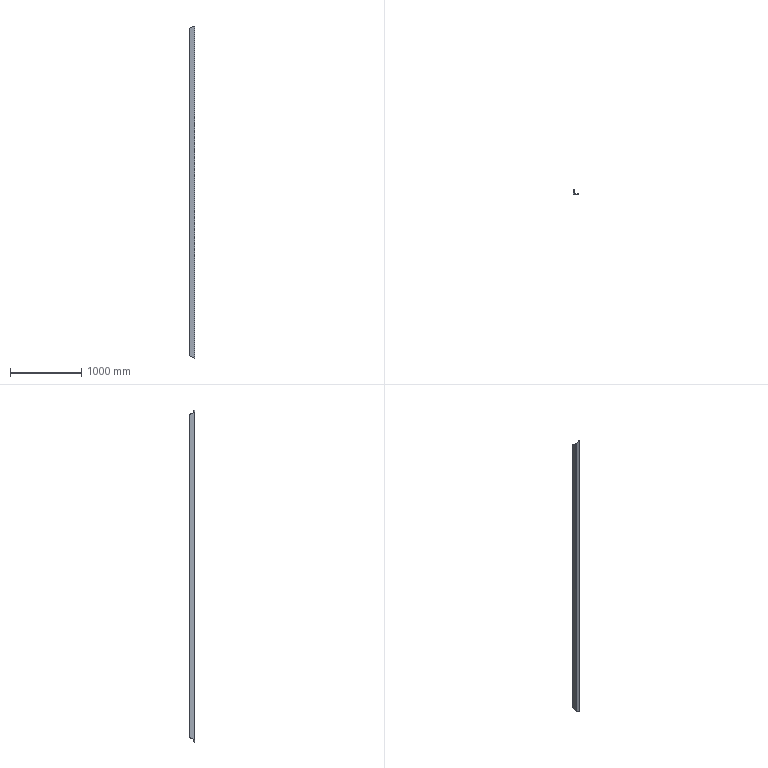Part | SolidWorks | features Extrusion 1, ICE 1 | 1 solid | 11 faces | box 70 x 70 x 4645 mm | volume 4877091 mm3 | plane 8 | cylinder 3 | commonest cylinder face diameters 6 x2 16 x1
STEP:
#1=CARTESIAN_POINT('',(5.,70.,4578.159));
#2=VERTEX_POINT('',#1);
#3=CARTESIAN_POINT('',(0.,70.,4575.683));
#4=VERTEX_POINT('',#3);
#5=CARTESIAN_POINT('',(31.579,70.,4591.318));
#6=DIRECTION('',(-0.8962,0.,-0.4437));
#7=VECTOR('',#6,1000.);
#8=LINE('',#5,#7);
#9=EDGE_CURVE('',#2,#4,#8,.T.);
#10=ORIENTED_EDGE('',*,*,#9,.F.);
#11=CARTESIAN_POINT('',(5.,70.,66.841));
#12=VERTEX_POINT('',#11);
#13=CARTESIAN_POINT('',(5.,70.,4645.));
#14=DIRECTION('',(0.,0.,-1.));
#15=VECTOR('',#14,1000.);
#16=LINE('',#13,#15);
#17=EDGE_CURVE('',#2,#12,#16,.T.);
#18=ORIENTED_EDGE('',*,*,#17,.T.);
#19=CARTESIAN_POINT('',(0.,70.,69.317));
#20=VERTEX_POINT('',#19);
#21=CARTESIAN_POINT('',(-1815.466,70.,968.193));
#22=DIRECTION('',(0.8962,0.,-0.4437));
#23=VECTOR('',#22,1000.);
#24=LINE('',#21,#23);
#25=EDGE_CURVE('',#20,#12,#24,.T.);
#26=ORIENTED_EDGE('',*,*,#25,.F.);
#27=CARTESIAN_POINT('',(0.,70.,4645.));
#28=DIRECTION('',(0.,0.,-1.));
#29=VECTOR('',#28,1000.);
#30=LINE('',#27,#29);
#31=EDGE_CURVE('',#4,#20,#30,.T.);
#32=ORIENTED_EDGE('',*,*,#31,.F.);
#33=EDGE_LOOP('',(#10,#18,#26,#32));
#34=FACE_OUTER_BOUND('',#33,.T.);
#35=CARTESIAN_POINT('',(5.,70.,4645.));
#36=DIRECTION('',(0.,-1.,0.));
#37=DIRECTION('',(0.,0.,-1.));
#38=AXIS2_PLACEMENT_3D('',#35,#36,#37);
#39=PLANE('',#38);
#40=ADVANCED_FACE('',(#34),#39,.F.);
#41=CARTESIAN_POINT('',(0.,0.,4610.341));
#42=VERTEX_POINT('',#41);
#43=CARTESIAN_POINT('',(0.,42.437,4589.33));
#44=DIRECTION('',(0.,-0.8962,0.4437));
#45=VECTOR('',#44,1000.);
#46=LINE('',#43,#45);
#47=EDGE_CURVE('',#4,#42,#46,.T.);
#48=ORIENTED_EDGE('',*,*,#47,.F.);
#49=ORIENTED_EDGE('',*,*,#31,.T.);
#50=CARTESIAN_POINT('',(0.,0.,34.659));
#51=VERTEX_POINT('',#50);
#52=CARTESIAN_POINT('',(0.,1889.482,970.181));
#53=DIRECTION('',(0.,0.8962,0.4437));
#54=VECTOR('',#53,1000.);
#55=LINE('',#52,#54);
#56=EDGE_CURVE('',#51,#20,#55,.T.);
#57=ORIENTED_EDGE('',*,*,#56,.F.);
#58=CARTESIAN_POINT('',(0.,0.,4645.));
#59=DIRECTION('',(0.,0.,-1.));
#60=VECTOR('',#59,1000.);
#61=LINE('',#58,#60);
#62=EDGE_CURVE('',#42,#51,#61,.T.);
#63=ORIENTED_EDGE('',*,*,#62,.F.);
#64=EDGE_LOOP('',(#48,#49,#57,#63));
#65=FACE_OUTER_BOUND('',#64,.T.);
#66=CARTESIAN_POINT('',(0.,70.,4645.));
#67=DIRECTION('',(1.,0.,0.));
#68=DIRECTION('',(0.,0.,-1.));
#69=AXIS2_PLACEMENT_3D('',#66,#67,#68);
#70=PLANE('',#69);
#71=ADVANCED_FACE('',(#65),#70,.F.);
#72=CARTESIAN_POINT('',(70.,0.,4645.));
#73=VERTEX_POINT('',#72);
#74=CARTESIAN_POINT('',(13.782,0.,4617.165));
#75=DIRECTION('',(0.8962,0.,0.4437));
#76=VECTOR('',#75,1000.);
#77=LINE('',#74,#76);
#78=EDGE_CURVE('',#42,#73,#77,.T.);
#79=ORIENTED_EDGE('',*,*,#78,.F.);
#80=ORIENTED_EDGE('',*,*,#62,.T.);
#81=CARTESIAN_POINT('',(70.,0.,0.));
#82=VERTEX_POINT('',#81);
#83=CARTESIAN_POINT('',(-1833.263,0.,942.347));
#84=DIRECTION('',(-0.8962,0.,0.4437));
#85=VECTOR('',#84,1000.);
#86=LINE('',#83,#85);
#87=EDGE_CURVE('',#82,#51,#86,.T.);
#88=ORIENTED_EDGE('',*,*,#87,.F.);
#89=CARTESIAN_POINT('',(70.,0.,4645.));
#90=DIRECTION('',(0.,0.,-1.));
#91=VECTOR('',#90,1000.);
#92=LINE('',#89,#91);
#93=EDGE_CURVE('',#73,#82,#92,.T.);
#94=ORIENTED_EDGE('',*,*,#93,.F.);
#95=EDGE_LOOP('',(#79,#80,#88,#94));
#96=FACE_OUTER_BOUND('',#95,.T.);
#97=CARTESIAN_POINT('',(0.,0.,4645.));
#98=DIRECTION('',(0.,1.,0.));
#99=DIRECTION('',(0.,0.,1.));
#100=AXIS2_PLACEMENT_3D('',#97,#98,#99);
#101=PLANE('',#100);
#102=ADVANCED_FACE('',(#96),#101,.F.);
#103=CARTESIAN_POINT('',(70.,5.,4642.524));
#104=VERTEX_POINT('',#103);
#105=CARTESIAN_POINT('',(70.,0.,4645.));
#106=DIRECTION('',(0.,0.8962,-0.4437));
#107=VECTOR('',#106,1000.);
#108=LINE('',#105,#107);
#109=EDGE_CURVE('',#73,#104,#108,.T.);
#110=ORIENTED_EDGE('',*,*,#109,.F.);
#111=ORIENTED_EDGE('',*,*,#93,.T.);
#112=CARTESIAN_POINT('',(70.,5.,2.476));
#113=VERTEX_POINT('',#112);
#114=CARTESIAN_POINT('',(70.,1847.045,914.512));
#115=DIRECTION('',(0.,-0.8962,-0.4437));
#116=VECTOR('',#115,1000.);
#117=LINE('',#114,#116);
#118=EDGE_CURVE('',#113,#82,#117,.T.);
#119=ORIENTED_EDGE('',*,*,#118,.F.);
#120=CARTESIAN_POINT('',(70.,5.,4645.));
#121=DIRECTION('',(0.,0.,-1.));
#122=VECTOR('',#121,1000.);
#123=LINE('',#120,#122);
#124=EDGE_CURVE('',#104,#113,#123,.T.);
#125=ORIENTED_EDGE('',*,*,#124,.F.);
#126=EDGE_LOOP('',(#110,#111,#119,#125));
#127=FACE_OUTER_BOUND('',#126,.T.);
#128=CARTESIAN_POINT('',(70.,0.,4645.));
#129=DIRECTION('',(-1.,0.,0.));
#130=DIRECTION('',(0.,0.,1.));
#131=AXIS2_PLACEMENT_3D('',#128,#129,#130);
#132=PLANE('',#131);
#133=ADVANCED_FACE('',(#127),#132,.F.);
#134=CARTESIAN_POINT('',(67.,8.,4639.554));
#135=VERTEX_POINT('',#134);
#136=CARTESIAN_POINT('',(70.,5.,4642.524));
#137=CARTESIAN_POINT('',(70.,6.757,4641.654));
#138=CARTESIAN_POINT('',(68.757,8.,4640.424));
#139=CARTESIAN_POINT('',(67.,8.,4639.554));
#140=(BOUNDED_CURVE()B_SPLINE_CURVE(3,(#136,#137,#138,#139),.UNSPECIFIED.,.F.,.F.)B_SPLINE_CURVE_WITH_KNOTS((4,4),(3.927,5.498),.UNSPECIFIED.)CURVE()GEOMETRIC_REPRESENTATION_ITEM()RATIONAL_B_SPLINE_CURVE((1.,0.8047,0.8047,1.))REPRESENTATION_ITEM(''));
#141=EDGE_CURVE('',#104,#135,#140,.T.);
#142=ORIENTED_EDGE('',*,*,#141,.F.);
#143=ORIENTED_EDGE('',*,*,#124,.T.);
#144=CARTESIAN_POINT('',(67.,8.,5.446));
#145=VERTEX_POINT('',#144);
#146=CARTESIAN_POINT('',(67.,8.,5.446));
#147=CARTESIAN_POINT('',(68.757,8.,4.576));
#148=CARTESIAN_POINT('',(70.,6.757,3.346));
#149=CARTESIAN_POINT('',(70.,5.,2.476));
#150=(BOUNDED_CURVE()B_SPLINE_CURVE(3,(#146,#147,#148,#149),.UNSPECIFIED.,.F.,.F.)B_SPLINE_CURVE_WITH_KNOTS((4,4),(3.927,5.498),.UNSPECIFIED.)CURVE()GEOMETRIC_REPRESENTATION_ITEM()RATIONAL_B_SPLINE_CURVE((1.,0.8047,0.8047,1.))REPRESENTATION_ITEM(''));
#151=EDGE_CURVE('',#145,#113,#150,.T.);
#152=ORIENTED_EDGE('',*,*,#151,.F.);
#153=CARTESIAN_POINT('',(67.,8.,4645.));
#154=DIRECTION('',(0.,0.,-1.));
#155=VECTOR('',#154,1000.);
#156=LINE('',#153,#155);
#157=EDGE_CURVE('',#135,#145,#156,.T.);
#158=ORIENTED_EDGE('',*,*,#157,.F.);
#159=EDGE_LOOP('',(#142,#143,#152,#158));
#160=FACE_OUTER_BOUND('',#159,.T.);
#161=CARTESIAN_POINT('',(67.,5.,4645.));
#162=DIRECTION('',(0.,0.,-1.));
#163=DIRECTION('',(-1.,0.,0.));
#164=AXIS2_PLACEMENT_3D('',#161,#162,#163);
#165=CYLINDRICAL_SURFACE('',#164,3.);
#166=ADVANCED_FACE('',(#160),#165,.T.);
#167=CARTESIAN_POINT('',(16.,8.,4614.302));
#168=VERTEX_POINT('',#167);
#169=CARTESIAN_POINT('',(69.166,8.,4640.626));
#170=DIRECTION('',(-0.8962,0.,-0.4437));
#171=VECTOR('',#170,1000.);
#172=LINE('',#169,#171);
#173=EDGE_CURVE('',#135,#168,#172,.T.);
#174=ORIENTED_EDGE('',*,*,#173,.F.);
#175=ORIENTED_EDGE('',*,*,#157,.T.);
#176=CARTESIAN_POINT('',(16.,8.,30.698));
#177=VERTEX_POINT('',#176);
#178=CARTESIAN_POINT('',(-1777.879,8.,918.886));
#179=DIRECTION('',(0.8962,0.,-0.4437));
#180=VECTOR('',#179,1000.);
#181=LINE('',#178,#180);
#182=EDGE_CURVE('',#177,#145,#181,.T.);
#183=ORIENTED_EDGE('',*,*,#182,.F.);
#184=CARTESIAN_POINT('',(16.,8.,4645.));
#185=DIRECTION('',(0.,0.,-1.));
#186=VECTOR('',#185,1000.);
#187=LINE('',#184,#186);
#188=EDGE_CURVE('',#168,#177,#187,.T.);
#189=ORIENTED_EDGE('',*,*,#188,.F.);
#190=EDGE_LOOP('',(#174,#175,#183,#189));
#191=FACE_OUTER_BOUND('',#190,.T.);
#192=CARTESIAN_POINT('',(67.,8.,4645.));
#193=DIRECTION('',(0.,-1.,0.));
#194=DIRECTION('',(1.,0.,0.));
#195=AXIS2_PLACEMENT_3D('',#192,#193,#194);
#196=PLANE('',#195);
#197=ADVANCED_FACE('',(#191),#196,.F.);
#198=CARTESIAN_POINT('',(8.,16.,4606.381));
#199=VERTEX_POINT('',#198);
#200=CARTESIAN_POINT('',(16.,8.,4614.302));
#201=CARTESIAN_POINT('',(11.314,8.,4611.982));
#202=CARTESIAN_POINT('',(8.,11.314,4608.701));
#203=CARTESIAN_POINT('',(8.,16.,4606.381));
#204=(BOUNDED_CURVE()B_SPLINE_CURVE(3,(#200,#201,#202,#203),.UNSPECIFIED.,.F.,.F.)B_SPLINE_CURVE_WITH_KNOTS((4,4),(3.927,5.498),.UNSPECIFIED.)CURVE()GEOMETRIC_REPRESENTATION_ITEM()RATIONAL_B_SPLINE_CURVE((1.,0.8047,0.8047,1.))REPRESENTATION_ITEM(''));
#205=EDGE_CURVE('',#168,#199,#204,.T.);
#206=ORIENTED_EDGE('',*,*,#205,.F.);
#207=ORIENTED_EDGE('',*,*,#188,.T.);
#208=CARTESIAN_POINT('',(8.,16.,38.619));
#209=VERTEX_POINT('',#208);
#210=CARTESIAN_POINT('',(8.,16.,38.619));
#211=CARTESIAN_POINT('',(8.,11.314,36.299));
#212=CARTESIAN_POINT('',(11.314,8.,33.018));
#213=CARTESIAN_POINT('',(16.,8.,30.698));
#214=(BOUNDED_CURVE()B_SPLINE_CURVE(3,(#210,#211,#212,#213),.UNSPECIFIED.,.F.,.F.)B_SPLINE_CURVE_WITH_KNOTS((4,4),(3.927,5.498),.UNSPECIFIED.)CURVE()GEOMETRIC_REPRESENTATION_ITEM()RATIONAL_B_SPLINE_CURVE((1.,0.8047,0.8047,1.))REPRESENTATION_ITEM(''));
#215=EDGE_CURVE('',#209,#177,#214,.T.);
#216=ORIENTED_EDGE('',*,*,#215,.F.);
#217=CARTESIAN_POINT('',(8.,16.,4645.));
#218=DIRECTION('',(0.,0.,-1.));
#219=VECTOR('',#218,1000.);
#220=LINE('',#217,#219);
#221=EDGE_CURVE('',#199,#209,#220,.T.);
#222=ORIENTED_EDGE('',*,*,#221,.F.);
#223=EDGE_LOOP('',(#206,#207,#216,#222));
#224=FACE_OUTER_BOUND('',#223,.T.);
#225=CARTESIAN_POINT('',(16.,16.,4645.));
#226=DIRECTION('',(0.,0.,-1.));
#227=DIRECTION('',(-1.,0.,0.));
#228=AXIS2_PLACEMENT_3D('',#225,#226,#227);
#229=CYLINDRICAL_SURFACE('',#228,8.);
#230=ADVANCED_FACE('',(#224),#229,.F.);
#231=CARTESIAN_POINT('',(8.,67.,4581.129));
#232=VERTEX_POINT('',#231);
#233=CARTESIAN_POINT('',(8.,0.6433,4613.984));
#234=DIRECTION('',(0.,0.8962,-0.4437));
#235=VECTOR('',#234,1000.);
#236=LINE('',#233,#235);
#237=EDGE_CURVE('',#199,#232,#236,.T.);
#238=ORIENTED_EDGE('',*,*,#237,.F.);
#239=ORIENTED_EDGE('',*,*,#221,.T.);
#240=CARTESIAN_POINT('',(8.,67.,63.871));
#241=VERTEX_POINT('',#240);
#242=CARTESIAN_POINT('',(8.,1847.688,945.528));
#243=DIRECTION('',(0.,-0.8962,-0.4437));
#244=VECTOR('',#243,1000.);
#245=LINE('',#242,#244);
#246=EDGE_CURVE('',#241,#209,#245,.T.);
#247=ORIENTED_EDGE('',*,*,#246,.F.);
#248=CARTESIAN_POINT('',(8.,67.,4645.));
#249=DIRECTION('',(0.,0.,-1.));
#250=VECTOR('',#249,1000.);
#251=LINE('',#248,#250);
#252=EDGE_CURVE('',#232,#241,#251,.T.);
#253=ORIENTED_EDGE('',*,*,#252,.F.);
#254=EDGE_LOOP('',(#238,#239,#247,#253));
#255=FACE_OUTER_BOUND('',#254,.T.);
#256=CARTESIAN_POINT('',(8.,16.,4645.));
#257=DIRECTION('',(-1.,0.,0.));
#258=DIRECTION('',(0.,-1.,0.));
#259=AXIS2_PLACEMENT_3D('',#256,#257,#258);
#260=PLANE('',#259);
#261=ADVANCED_FACE('',(#255),#260,.F.);
#262=CARTESIAN_POINT('',(8.,67.,4581.129));
#263=CARTESIAN_POINT('',(8.,68.757,4580.259));
#264=CARTESIAN_POINT('',(6.757,70.,4579.029));
#265=CARTESIAN_POINT('',(5.,70.,4578.159));
#266=(BOUNDED_CURVE()B_SPLINE_CURVE(3,(#262,#263,#264,#265),.UNSPECIFIED.,.F.,.F.)B_SPLINE_CURVE_WITH_KNOTS((4,4),(3.927,5.498),.UNSPECIFIED.)CURVE()GEOMETRIC_REPRESENTATION_ITEM()RATIONAL_B_SPLINE_CURVE((1.,0.8047,0.8047,1.))REPRESENTATION_ITEM(''));
#267=EDGE_CURVE('',#232,#2,#266,.T.);
#268=ORIENTED_EDGE('',*,*,#267,.F.);
#269=ORIENTED_EDGE('',*,*,#252,.T.);
#270=CARTESIAN_POINT('',(5.,70.,66.841));
#271=CARTESIAN_POINT('',(6.757,70.,65.971));
#272=CARTESIAN_POINT('',(8.,68.757,64.741));
#273=CARTESIAN_POINT('',(8.,67.,63.871));
#274=(BOUNDED_CURVE()B_SPLINE_CURVE(3,(#270,#271,#272,#273),.UNSPECIFIED.,.F.,.F.)B_SPLINE_CURVE_WITH_KNOTS((4,4),(3.927,5.498),.UNSPECIFIED.)CURVE()GEOMETRIC_REPRESENTATION_ITEM()RATIONAL_B_SPLINE_CURVE((1.,0.8047,0.8047,1.))REPRESENTATION_ITEM(''));
#275=EDGE_CURVE('',#12,#241,#274,.T.);
#276=ORIENTED_EDGE('',*,*,#275,.F.);
#277=ORIENTED_EDGE('',*,*,#17,.F.);
#278=EDGE_LOOP('',(#268,#269,#276,#277));
#279=FACE_OUTER_BOUND('',#278,.T.);
#280=CARTESIAN_POINT('',(5.,67.,4645.));
#281=DIRECTION('',(0.,0.,-1.));
#282=DIRECTION('',(-1.,0.,0.));
#283=AXIS2_PLACEMENT_3D('',#280,#281,#282);
#284=CYLINDRICAL_SURFACE('',#283,3.);
#285=ADVANCED_FACE('',(#279),#284,.T.);
#286=ORIENTED_EDGE('',*,*,#25,.T.);
#287=ORIENTED_EDGE('',*,*,#275,.T.);
#288=ORIENTED_EDGE('',*,*,#246,.T.);
#289=ORIENTED_EDGE('',*,*,#215,.T.);
#290=ORIENTED_EDGE('',*,*,#182,.T.);
#291=ORIENTED_EDGE('',*,*,#151,.T.);
#292=ORIENTED_EDGE('',*,*,#118,.T.);
#293=ORIENTED_EDGE('',*,*,#87,.T.);
#294=ORIENTED_EDGE('',*,*,#56,.T.);
#295=EDGE_LOOP('',(#286,#287,#288,#289,#290,#291,#292,#293,#294));
#296=FACE_OUTER_BOUND('',#295,.T.);
#297=CARTESIAN_POINT('',(105.,35.,0.));
#298=DIRECTION('',(-0.4056,0.4056,-0.8192));
#299=DIRECTION('',(0.,0.8962,0.4437));
#300=AXIS2_PLACEMENT_3D('',#297,#298,#299);
#301=PLANE('',#300);
#302=ADVANCED_FACE('',(#296),#301,.T.);
#303=ORIENTED_EDGE('',*,*,#9,.T.);
#304=ORIENTED_EDGE('',*,*,#47,.T.);
#305=ORIENTED_EDGE('',*,*,#78,.T.);
#306=ORIENTED_EDGE('',*,*,#109,.T.);
#307=ORIENTED_EDGE('',*,*,#141,.T.);
#308=ORIENTED_EDGE('',*,*,#173,.T.);
#309=ORIENTED_EDGE('',*,*,#205,.T.);
#310=ORIENTED_EDGE('',*,*,#237,.T.);
#311=ORIENTED_EDGE('',*,*,#267,.T.);
#312=EDGE_LOOP('',(#303,#304,#305,#306,#307,#308,#309,#310,#311));
#313=FACE_OUTER_BOUND('',#312,.T.);
#314=CARTESIAN_POINT('',(35.,105.,4575.683));
#315=DIRECTION('',(-0.4056,0.4056,0.8192));
#316=DIRECTION('',(0.,-0.8962,0.4437));
#317=AXIS2_PLACEMENT_3D('',#314,#315,#316);
#318=PLANE('',#317);
#319=ADVANCED_FACE('',(#313),#318,.T.);
#320=CLOSED_SHELL('',(#40,#71,#102,#133,#166,#197,#230,#261,#285,#302,#319));
#321=MANIFOLD_SOLID_BREP('',#320);
#322=CARTESIAN_POINT('',(0.,0.,0.));
#323=DIRECTION('',(0.,0.,1.));
#324=DIRECTION('',(1.,0.,0.));
#325=AXIS2_PLACEMENT_3D('',#322,#323,#324);
#326=(LENGTH_UNIT()NAMED_UNIT(*)SI_UNIT(.MILLI.,.METRE.));
#327=UNCERTAINTY_MEASURE_WITH_UNIT(LENGTH_MEASURE(0.00001),#326,'','');
#328=(NAMED_UNIT(*)PLANE_ANGLE_UNIT()SI_UNIT($,.RADIAN.));
#329=(NAMED_UNIT(*)SI_UNIT($,.STERADIAN.)SOLID_ANGLE_UNIT());
#330=(GEOMETRIC_REPRESENTATION_CONTEXT(3)GLOBAL_UNCERTAINTY_ASSIGNED_CONTEXT((#327))GLOBAL_UNIT_ASSIGNED_CONTEXT((#326,#328,#329))REPRESENTATION_CONTEXT('',''));
#331=ADVANCED_BREP_SHAPE_REPRESENTATION('',(#321,#325),#330);